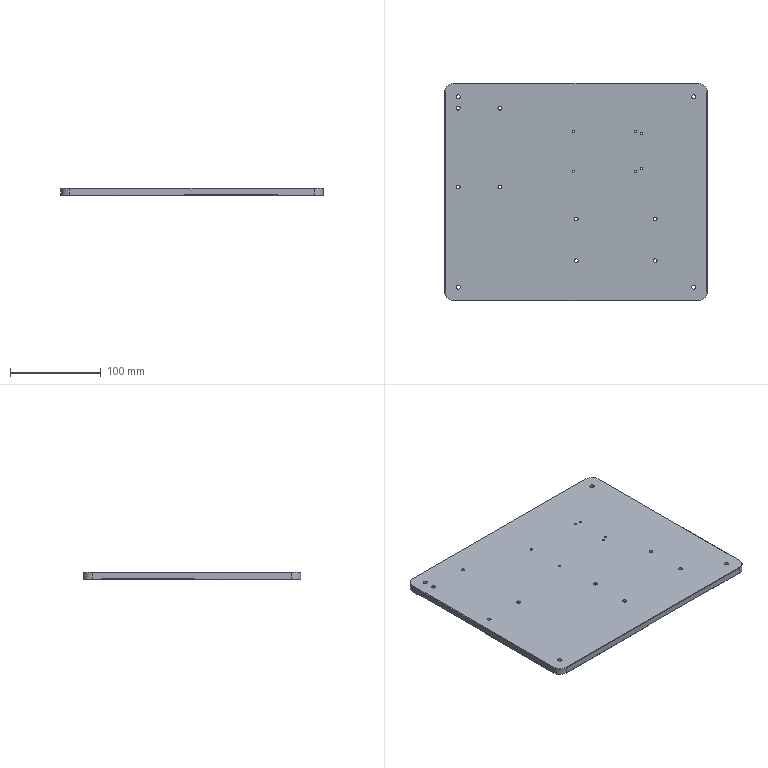CAM job | NX | 3-axis milling, drilling | part box 290 x 240 x 8 mm | stock box 295 x 245 x 8 mm
Tools:
number,name,description,diameter,corner_radius,flute_length,length,flutes
18,D2,平底铣刀-粗,2.0,0.0,50.0,75.0,2
4,D4,平底铣刀-粗,4.0,0.0,25.0,75.0,2
9,D10,平底铣刀-粗,10.0,0.0,35.0,75.0,2
17,D2-J,平底铣刀-精,2.0,0.0,50.0,75.0,2
7,D6-J,平底铣刀-精,6.0,0.0,25.0,75.0,2
2,D6倒角刀,倒角刀,6.0,0.0,3.0,25.0,2
20,M3X0.5,丝锥,2.5,0.0,35.0,50.0,2
22,M5X0.8,丝锥,4.2,0.0,35.0,50.0,2
12,ZT2.5,钻头,2.5,0.0,35.0,50.0,2
11,ZT4.5,钻头,4.5,0.0,35.0,50.0,2
14,钻头4.2,Twist Drill 4.2 mm,4.2,0.0,41.0,41.738,2
Operations:
program,operation,operation_type,tool,method,geometry_group,spindle_rpm,surface_speed,feed_per_tooth,feed_cut,feed_plunge,cut_length_mm,path_length_mm,cut_time_min,machine_time_min
B,打点-深0.8,Operation,D6倒角刀,NONE,W-B,8000.0,150.796,0.0312,500.0,90.0,32.4,1070.475,0.0648,0.1686
B,通孔-M3螺纹底孔,Operation,ZT2.5,NONE,W-B,3000.0,23.562,0.05,300.0,90.0,78.507,367.62,0.2617,0.2906
B,通孔-M5螺纹底孔,Operation,钻头4.2,NONE,W-B,3000.0,39.584,0.0583,350.0,90.0,122.094,740.619,0.3488,0.4107
B,通孔-5-6,Operation,ZT4.5,NONE,W-B,3000.0,42.411,0.025,150.0,90.0,31.008,785.022,0.2067,0.2821
B,钻倒角_4,Operation,D6倒角刀,METHOD,W-B,8000.0,150.796,0.0312,500.0,0.0,28.5,278.956,0.057,0.082
B,铣倒角_2,PlanarMilling,D6倒角刀,METHOD,W-B,8000.0,150.796,0.0312,500.0,100.0,144.163,921.07,0.2883,0.366
B,铣倒角_3,PlanarMilling,D6倒角刀,METHOD,W-B,8000.0,150.796,0.0312,500.0,100.0,69.412,913.414,0.1388,0.2232
B,底壁铣倒角_COPY_1,VolumeBased25DMillingOperation,D6倒角刀,爬面_倒角-切深0-步距G,W-B,6500.0,122.519,0.1154,1500.0,100.0,1054.34,1093.739,0.7029,0.7068
B,通孔-攻牙M3,Operation,M3X0.5,METHOD,W-B,800.0,6.283,0.0003,0.5,90.0,62.0,334.607,124.0,124.027
B,通孔-攻牙M5,Operation,M5X0.8,METHOD,W-B,500.0,6.597,0.0008,0.8,90.0,92.0,680.43,115.0,115.059
A,打点,Operation,D6倒角刀,METHOD,W-A,3000.0,56.549,0.0333,200.0,0.0,35.0,997.455,0.175,0.2712
A,打点_2,Operation,D6倒角刀,METHOD,W-A,3000.0,56.549,0.0333,200.0,0.0,8.0,215.381,0.04,0.0607
A,打孔_2,Operation,ZT2.5,METHOD,W-A,3000.0,23.562,0.025,150.0,0.0,17.4,114.813,0.116,0.1257
A,打孔_5,Operation,ZT4.5,METHOD,W-A,2500.0,35.343,0.024,120.0,0.0,34.8,792.607,0.29,0.3658
A,底壁粗_1,VolumeBased25DMillingOperation,D10,METHOD,W-A,6000.0,113.0,0.2083,3500.0,100.0,3182.216,3272.465,0.9092,0.9182
A,底壁粗_2,VolumeBased25DMillingOperation,D10,METHOD,W-A,6000.0,113.0,0.2083,3500.0,100.0,2404.383,2482.71,0.687,0.6948
A,孔粗_1,CylinderMilling,D4,METHOD,W-A,6000.0,75.398,0.15,1800.0,100.0,752.129,1609.329,0.4178,0.5036
A,孔侧_1,CylinderMilling,D4,METHOD,W-A,6000.0,75.398,0.05,600.0,100.0,70.071,946.871,0.1168,0.2045
A,底壁铣螺旋开粗-小_COPY,VolumeBased25DMillingOperation,D2,分层开粗-切深K-步距G,W-A,8000.0,50.264,0.0312,500.0,100.0,641.894,767.021,1.284,1.296
A,清角D4,ZLevelMilling,D2-J,METHOD,W-A,9000.0,56.549,0.0833,1500.0,80.0,383.489,865.12,0.2567,0.3049
A,外形粗_2,VolumeBased25DMillingOperation,D10,METHOD,W-A,6000.0,188.0,0.25,4000.0,80.0,19349.271,19395.271,4.837,4.842
A,底精_1,VolumeBased25DMillingOperation,D6-J,METHOD,W-A,6000.0,113.0,0.2083,1200.0,100.0,2520.386,2561.386,2.1,2.104
A,底精_2,VolumeBased25DMillingOperation,D6-J,METHOD,W-A,6000.0,113.0,0.2083,1200.0,100.0,1817.5,1858.5,1.515,1.519
A,仅选体,SurfaceContour,D6倒角刀,METHOD,W-A,6000.0,113.0,0.125,1200.0,100.0,787.106,1613.176,0.6559,0.7385
A,钻倒角_1,Operation,D6倒角刀,METHOD,W-A,5000.0,94.248,0.015,150.0,0.0,19.0,243.621,0.1267,0.1491
A,钻倒角_2,Operation,D6倒角刀,METHOD,W-A,5000.0,94.248,0.015,150.0,0.0,10.6,103.315,0.0707,0.0799
A,钻倒角_3,Operation,D6倒角刀,METHOD,W-A,5000.0,94.248,0.015,150.0,0.0,45.6,604.113,0.304,0.3599
A,铣倒角_1,PlanarMilling,D6倒角刀,METHOD,W-A,6000.0,113.097,0.05,600.0,100.0,83.855,935.865,0.1398,0.225
A,底壁铣倒角_COPY,VolumeBased25DMillingOperation,D6倒角刀,爬面_倒角-切深0-步距G,W-A,6500.0,122.519,0.1154,1500.0,100.0,1054.325,1093.725,0.7029,0.7068
A,底壁铣螺旋精光-小_COPY,VolumeBased25DMillingOperation,D2-J,螺旋精光-切深K-步距G,W-A,8000.0,50.266,0.0125,200.0,100.0,111.832,237.227,0.5592,0.5717
A,底侧精_3,VolumeBased25DMillingOperation,D6-J,METHOD,W-A,6000.0,113.0,0.2083,1200.0,100.0,307.315,348.305,0.2561,0.2602
A,底侧精_4,VolumeBased25DMillingOperation,D6-J,METHOD,W-A,6000.0,113.0,0.2083,1200.0,100.0,248.742,289.732,0.2073,0.2114
A,外形半精_2,VolumeBased25DMillingOperation,D6-J,METHOD,W-A,6000.0,113.0,0.0833,1000.0,100.0,1066.687,1120.687,1.067,1.072
A,外形精_2,VolumeBased25DMillingOperation,D6-J,METHOD,W-A,6000.0,113.0,0.0833,1000.0,100.0,1066.487,1121.087,1.067,1.072